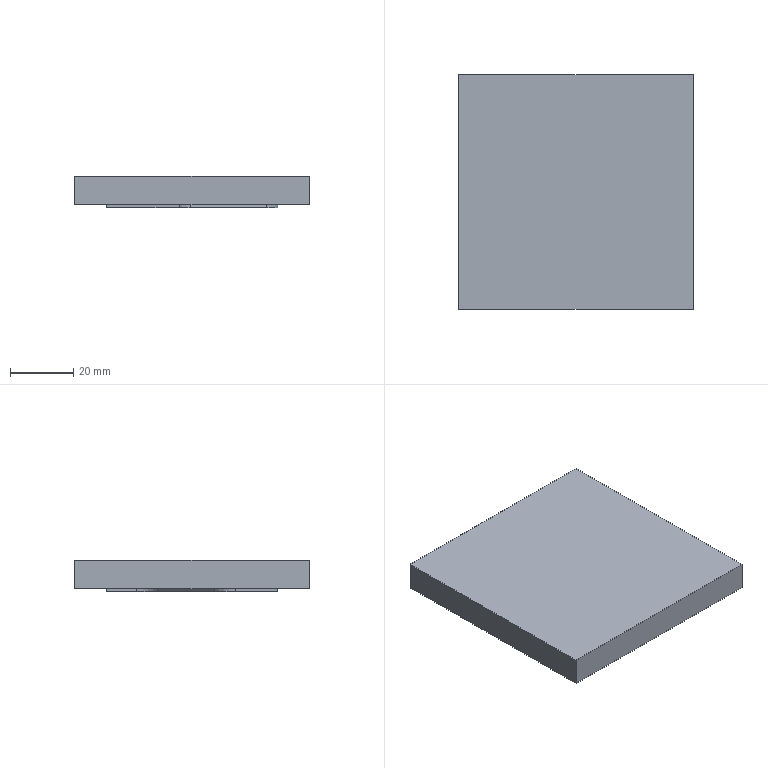NC program | NX | posted with a generic post | part box 74 x 74 x 10 mm
Whole program:
N10 G17 G21 G94 G90
(ZLEVEL_PROFILE_1_COPY_COPY_COPY , TOOL : D1.5)
N12 T19 M6
N14 G54
N16 G17 G0 G90 X3.472 Y4.658 B0. C0. S7500 M3
N18 G43 Z30. H19
N20 Z0.145
N22 G94 G1 X3.468 Y4.656 Z0.108 F1000.
N24 X3.459 Y4.648 Z0.076
N26 X3.445 Y4.635 Z0.047
N28 X3.427 Y4.614 Z0.022
N30 X3.406 Y4.587 Z0.
N32 X3.383 Y4.552 Z-0.019
N34 X3.359 Y4.508 Z-0.035
N36 X3.336 Y4.455 Z-0.048
N38 X3.313 Y4.392 Z-0.059
N40 X3.292 Y4.319 Z-0.067
N42 X3.274 Y4.235 Z-0.073
N44 X3.26 Y4.139 Z-0.077
N46 X3.251 Y4.03 Z-0.079
N48 X3.248 Y3.908 Z-0.08
N50 X3.25 Y2.469 F800.
N52 Y-0.25
N54 X15.75
N56 Y-0.18
N58 Y0.231
N60 X15.701 Y0.254
N62 X14.11 Y0.25
N64 X4.5
N66 G2 X3.75 Y1. R0.75
N68 G1 Y2.5
N70 X3.753 Y3.908
N72 X3.748 Y3.959 Z-0.081
N74 X3.735 Y4.003 Z-0.082
N76 X3.715 Y4.04 Z-0.085
N78 X3.69 Y4.071 Z-0.088
N80 X3.631 Y4.116 Z-0.097
N82 X3.549 Y4.15 Z-0.111
N84 X3.5 Y4.156 Z-0.12
N86 X3.452 Y4.15 Z-0.129
N88 X3.37 Y4.116 Z-0.143
N90 X3.311 Y4.071 Z-0.152
N92 X3.286 Y4.04 Z-0.155
N94 X3.266 Y4.003 Z-0.158
N96 X3.253 Y3.959 Z-0.159
N98 X3.248 Y3.908 Z-0.16
N100 X3.25 Y2.469
N102 Y-0.25
N104 X15.75
N106 Y-0.18
N108 Y0.231
N110 X15.701 Y0.254
N112 X14.11 Y0.25
N114 X4.5
N116 G2 X3.75 Y1. R0.75
N118 G1 Y2.5
N120 X3.753 Y3.908
N122 X3.748 Y3.959 Z-0.161
N124 X3.735 Y4.003 Z-0.162
N126 X3.715 Y4.04 Z-0.165
N128 X3.69 Y4.071 Z-0.168
N130 X3.631 Y4.116 Z-0.177
N132 X3.549 Y4.15 Z-0.191
N134 X3.5 Y4.156 Z-0.2
N136 X3.452 Y4.15 Z-0.209
N138 X3.37 Y4.116 Z-0.223
N140 X3.311 Y4.071 Z-0.232
N142 X3.286 Y4.04 Z-0.235
N144 X3.266 Y4.003 Z-0.238
N146 X3.253 Y3.959 Z-0.239
N148 X3.248 Y3.908 Z-0.24
N150 X3.25 Y2.469
N152 Y-0.25
N154 X15.75
N156 Y-0.18
N158 Y0.231
N160 X15.701 Y0.254
N162 X14.11 Y0.25
N164 X4.5
N166 G2 X3.75 Y1. R0.75
N168 G1 Y2.5
N170 X3.753 Y3.908
N172 X3.748 Y3.959 Z-0.241
N174 X3.735 Y4.003 Z-0.242
N176 X3.715 Y4.04 Z-0.245
N178 X3.69 Y4.071 Z-0.248
N180 X3.631 Y4.116 Z-0.257
N182 X3.549 Y4.15 Z-0.271
N184 X3.5 Y4.156 Z-0.28
N186 X3.452 Y4.15 Z-0.289
N188 X3.37 Y4.116 Z-0.303
N190 X3.311 Y4.071 Z-0.312
N192 X3.286 Y4.04 Z-0.315
N194 X3.266 Y4.003 Z-0.318
N196 X3.253 Y3.959 Z-0.319
N198 X3.248 Y3.908 Z-0.32
N200 X3.25 Y2.469
N202 Y-0.25
N204 X15.75
N206 Y-0.18
N208 Y0.231
N210 X15.701 Y0.254
N212 X14.11 Y0.25
N214 X4.5
N216 G2 X3.75 Y1. R0.75
N218 G1 Y2.5
N220 X3.753 Y3.908
N222 X3.748 Y3.959 Z-0.321
N224 X3.735 Y4.003 Z-0.322
N226 X3.715 Y4.04 Z-0.325
N228 X3.69 Y4.071 Z-0.328
N230 X3.631 Y4.116 Z-0.337
N232 X3.549 Y4.15 Z-0.351
N234 X3.5 Y4.156 Z-0.36
N236 X3.452 Y4.15 Z-0.369
N238 X3.37 Y4.116 Z-0.383
N240 X3.311 Y4.071 Z-0.392
N242 X3.286 Y4.04 Z-0.395
N244 X3.266 Y4.003 Z-0.398
N246 X3.253 Y3.959 Z-0.399
N248 X3.248 Y3.908 Z-0.4
N250 X3.25 Y2.469
N252 Y-0.25
N254 X15.75
N256 Y-0.18
N258 Y0.231
N260 X15.701 Y0.254
N262 X14.11 Y0.25
N264 X4.5
N266 G2 X3.75 Y1. R0.75
N268 G1 Y2.5
N270 X3.753 Y3.908
N272 X3.748 Y3.959 Z-0.401
N274 X3.735 Y4.003 Z-0.402
N276 X3.715 Y4.04 Z-0.405
N278 X3.69 Y4.071 Z-0.408
N280 X3.631 Y4.116 Z-0.417
N282 X3.549 Y4.15 Z-0.431
N284 X3.5 Y4.156 Z-0.44
N286 X3.452 Y4.15 Z-0.449
N288 X3.37 Y4.116 Z-0.463
N290 X3.311 Y4.071 Z-0.472
N292 X3.286 Y4.04 Z-0.475
N294 X3.266 Y4.003 Z-0.478
N296 X3.253 Y3.959 Z-0.479
N298 X3.248 Y3.908 Z-0.48
N300 X3.25 Y2.469
N302 Y-0.25
N304 X15.75
N306 Y-0.18
N308 Y0.231
N310 X15.701 Y0.254
N312 X14.11 Y0.25
N314 X4.5
N316 G2 X3.75 Y1. R0.75
N318 G1 Y2.5
N320 X3.753 Y3.908
N322 X3.748 Y3.959 Z-0.481
N324 X3.735 Y4.003 Z-0.482
N326 X3.715 Y4.04 Z-0.485
N328 X3.69 Y4.071 Z-0.488
N330 X3.631 Y4.116 Z-0.497
N332 X3.549 Y4.15 Z-0.511
N334 X3.5 Y4.156 Z-0.52
N336 X3.452 Y4.15 Z-0.529
N338 X3.37 Y4.116 Z-0.543
N340 X3.311 Y4.071 Z-0.552
N342 X3.286 Y4.04 Z-0.555
N344 X3.266 Y4.003 Z-0.558
N346 X3.253 Y3.959 Z-0.559
N348 X3.248 Y3.908 Z-0.56
N350 X3.25 Y2.469
N352 Y-0.25
N354 X15.75
N356 Y-0.18
N358 Y0.231
N360 X15.701 Y0.254
N362 X14.11 Y0.25
N364 X4.5
N366 G2 X3.75 Y1. R0.75
N368 G1 Y2.5
N370 X3.753 Y3.908
N372 X3.748 Y3.959 Z-0.561
N374 X3.735 Y4.003 Z-0.562
N376 X3.715 Y4.04 Z-0.565
N378 X3.69 Y4.071 Z-0.568
N380 X3.631 Y4.116 Z-0.577
N382 X3.549 Y4.15 Z-0.591
N384 X3.5 Y4.156 Z-0.6
N386 X3.452 Y4.15 Z-0.609
N388 X3.37 Y4.116 Z-0.623
N390 X3.311 Y4.071 Z-0.632
N392 X3.286 Y4.04 Z-0.635
N394 X3.266 Y4.003 Z-0.638
N396 X3.253 Y3.959 Z-0.639
N398 X3.248 Y3.908 Z-0.64
N400 X3.25 Y2.469
N402 Y-0.25
N404 X15.75
N406 Y-0.18
N408 Y0.231
N410 X15.701 Y0.254
N412 X14.11 Y0.25
N414 X4.5
N416 G2 X3.75 Y1. R0.75
N418 G1 Y2.5
N420 X3.753 Y3.908
N422 X3.748 Y3.959 Z-0.641
N424 X3.735 Y4.003 Z-0.642
N426 X3.715 Y4.04 Z-0.645
N428 X3.69 Y4.071 Z-0.648
N430 X3.631 Y4.116 Z-0.657
N432 X3.549 Y4.15 Z-0.671
N434 X3.5 Y4.156 Z-0.68
N436 X3.452 Y4.15 Z-0.689
N438 X3.37 Y4.116 Z-0.703
N440 X3.311 Y4.071 Z-0.712
N442 X3.286 Y4.04 Z-0.715
N444 X3.266 Y4.003 Z-0.718
N446 X3.253 Y3.959 Z-0.719
N448 X3.248 Y3.908 Z-0.72
N450 X3.25 Y2.469
N452 Y-0.25
N454 X15.75
N456 Y-0.18
N458 Y0.231
N460 X15.701 Y0.254
N462 X14.11 Y0.25
N464 X4.5
N466 G2 X3.75 Y1. R0.75
N468 G1 Y2.5
N470 X3.753 Y3.908
N472 X3.748 Y3.959 Z-0.721
N474 X3.735 Y4.003 Z-0.722
N476 X3.715 Y4.04 Z-0.725
N478 X3.69 Y4.071 Z-0.728
N480 X3.631 Y4.116 Z-0.737
N482 X3.549 Y4.15 Z-0.751
N484 X3.5 Y4.156 Z-0.76
N486 X3.452 Y4.15 Z-0.769
N488 X3.37 Y4.116 Z-0.783
N490 X3.311 Y4.071 Z-0.792
N492 X3.286 Y4.04 Z-0.795
N494 X3.266 Y4.003 Z-0.798
N496 X3.253 Y3.959 Z-0.799
N498 X3.248 Y3.908 Z-0.8
N500 X3.25 Y2.469
N502 Y-0.25
N504 X15.75
N506 Y-0.18
N508 Y0.231
N510 X15.701 Y0.253
N512 X14.11 Y0.25
N514 X4.5
N516 G2 X3.75 Y1. R0.75
N518 G1 Y2.5
N520 X3.753 Y3.908
N522 X3.748 Y3.959 Z-0.801
N524 X3.735 Y4.003 Z-0.802
N526 X3.715 Y4.04 Z-0.805
N528 X3.69 Y4.071 Z-0.808
N530 X3.631 Y4.116 Z-0.817
N532 X3.549 Y4.15 Z-0.831
N534 X3.5 Y4.156 Z-0.84
N536 X3.452 Y4.15 Z-0.849
N538 X3.37 Y4.116 Z-0.863
N540 X3.311 Y4.07 Z-0.872
N542 X3.286 Y4.04 Z-0.875
N544 X3.266 Y4.003 Z-0.878
N546 X3.253 Y3.959 Z-0.879
N548 X3.248 Y3.908 Z-0.88
N550 X3.25 Y2.469
N552 Y-0.25
N554 X15.75
N556 Y-0.18
N558 Y0.231
N560 X15.701 Y0.253
N562 X14.11 Y0.25
N564 X4.5
N566 G2 X3.75 Y1. R0.75
N568 G1 Y2.5
N570 X3.753 Y3.908
N572 X3.748 Y3.959 Z-0.881
N574 X3.735 Y4.003 Z-0.882
N576 X3.715 Y4.04 Z-0.885
N578 X3.69 Y4.07 Z-0.888
N580 X3.631 Y4.116 Z-0.897
N582 X3.549 Y4.15 Z-0.911
N584 X3.5 Y4.156 Z-0.92
N586 X3.452 Y4.15 Z-0.929
N588 X3.37 Y4.116 Z-0.943
N590 X3.311 Y4.07 Z-0.952
N592 X3.286 Y4.04 Z-0.955
N594 X3.266 Y4.003 Z-0.958
N596 X3.253 Y3.959 Z-0.959
N598 X3.248 Y3.908 Z-0.96
N600 X3.25 Y2.469
N602 Y-0.25
N604 X15.75
N606 Y-0.18
N608 Y0.231
N610 X15.701 Y0.253
N612 X14.11 Y0.25
N614 X4.5
N616 G2 X3.75 Y1. R0.75
N618 G1 Y2.5
N620 X3.752 Y3.908
N622 X3.748 Y3.959 Z-0.961
N624 X3.735 Y4.003 Z-0.962
N626 X3.715 Y4.04 Z-0.965
N628 X3.69 Y4.07 Z-0.968
N630 X3.631 Y4.116 Z-0.977
N632 X3.549 Y4.15 Z-0.991
N634 X3.5 Y4.156 Z-1.
N636 X3.452 Y4.15 Z-1.009
N638 X3.37 Y4.116 Z-1.023
N640 X3.311 Y4.07 Z-1.032
N642 X3.286 Y4.04 Z-1.035
N644 X3.266 Y4.003 Z-1.038
N646 X3.253 Y3.959 Z-1.039
N648 X3.248 Y3.908 Z-1.04
N650 X3.25 Y2.469
N652 Y-0.25
N654 X15.75
N656 Y-0.18
N658 Y0.231
N660 X15.701 Y0.253
N662 X14.11 Y0.25
N664 X4.5
N666 G2 X3.75 Y1. R0.75
N668 G1 Y2.5
N670 X3.752 Y3.908
N672 X3.748 Y3.959 Z-1.041
N674 X3.735 Y4.003 Z-1.042
N676 X3.715 Y4.04 Z-1.045
N678 X3.69 Y4.07 Z-1.048
N680 X3.631 Y4.116 Z-1.057
N682 X3.549 Y4.15 Z-1.071
N684 X3.5 Y4.155 Z-1.08
N686 X3.452 Y4.15 Z-1.089
N688 X3.37 Y4.116 Z-1.103
N690 X3.311 Y4.07 Z-1.112
N692 X3.286 Y4.04 Z-1.115
N694 X3.266 Y4.003 Z-1.118
N696 X3.253 Y3.959 Z-1.119
N698 X3.248 Y3.908 Z-1.12
N700 X3.25 Y2.469
N702 Y-0.25
N704 X15.75
N706 Y-0.18
N708 Y0.231
N710 X15.701 Y0.253
N712 X14.11 Y0.25
N714 X4.5
N716 G2 X3.75 Y1. R0.75
N718 G1 Y2.5
N720 X3.752 Y3.908
N722 X3.748 Y3.959 Z-1.121
N724 X3.735 Y4.003 Z-1.122
N726 X3.715 Y4.04 Z-1.125
N728 X3.69 Y4.07 Z-1.128
N730 X3.631 Y4.116 Z-1.137
N732 X3.549 Y4.149 Z-1.151
N734 X3.5 Y4.155 Z-1.16
N736 X3.452 Y4.149 Z-1.169
N738 X3.37 Y4.116 Z-1.183
N740 X3.311 Y4.07 Z-1.192
N742 X3.286 Y4.04 Z-1.195
N744 X3.266 Y4.003 Z-1.198
N746 X3.253 Y3.959 Z-1.199
N748 X3.248 Y3.908 Z-1.2
N750 X3.25 Y2.469
N752 Y-0.25
N754 X15.75
N756 Y-0.18
N758 Y0.231
N760 X15.701 Y0.253
N762 X14.11 Y0.25
N764 X4.5
N766 G2 X3.75 Y1. R0.75
N768 G1 Y2.5
N770 X3.752 Y3.908
N772 X3.748 Y3.959 Z-1.201
N774 X3.735 Y4.003 Z-1.202
N776 X3.715 Y4.04 Z-1.205
N778 X3.69 Y4.07 Z-1.208
N780 X3.631 Y4.116 Z-1.217
N782 X3.549 Y4.149 Z-1.231
N784 X3.5 Y4.155 Z-1.24
N786 X3.452 Y4.149 Z-1.249
N788 X3.37 Y4.116 Z-1.263
N790 X3.311 Y4.07 Z-1.272
N792 X3.286 Y4.04 Z-1.275
N794 X3.266 Y4.003 Z-1.278
N796 X3.253 Y3.959 Z-1.279
N798 X3.248 Y3.908 Z-1.28
N800 X3.25 Y2.469
N802 Y-0.25
N804 X15.75
N806 Y-0.18
N808 Y0.231
N810 X15.701 Y0.253
N812 X14.11 Y0.25
N814 X4.5
N816 G2 X3.75 Y1. R0.75
N818 G1 Y2.5
N820 X3.752 Y3.908
N822 X3.748 Y3.959 Z-1.281
N824 X3.735 Y4.003 Z-1.282
N826 X3.715 Y4.04 Z-1.285
N828 X3.69 Y4.07 Z-1.288
N830 X3.631 Y4.116 Z-1.297
N832 X3.549 Y4.149 Z-1.311
N834 X3.5 Y4.155 Z-1.32
N836 X3.452 Y4.149 Z-1.329
N838 X3.37 Y4.116 Z-1.343
N840 X3.311 Y4.07 Z-1.352
N842 X3.286 Y4.04 Z-1.355
N844 X3.266 Y4.003 Z-1.358
N846 X3.253 Y3.959 Z-1.359
N848 X3.248 Y3.908 Z-1.36
N850 X3.25 Y2.469
N852 Y-0.25
N854 X15.75
N856 Y-0.18
N858 Y0.231
N860 X15.701 Y0.253
N862 X14.11 Y0.25
N864 X4.5
N866 G2 X3.75 Y1. R0.75
N868 G1 Y2.5
N870 X3.752 Y3.908
N872 X3.748 Y3.959 Z-1.361
N874 X3.734 Y4.003 Z-1.362
N876 X3.715 Y4.04 Z-1.365
N878 X3.69 Y4.07 Z-1.368
N880 X3.631 Y4.116 Z-1.377
N882 X3.549 Y4.149 Z-1.391
N884 X3.5 Y4.155 Z-1.4
N886 X3.452 Y4.149 Z-1.409
N888 X3.37 Y4.116 Z-1.423
N890 X3.311 Y4.07 Z-1.432
N892 X3.286 Y4.04 Z-1.435
N894 X3.266 Y4.003 Z-1.438
N896 X3.253 Y3.959 Z-1.439
N898 X3.248 Y3.908 Z-1.44
N900 X3.25 Y2.469
N902 Y-0.25
N904 X15.75
N906 Y-0.18
N908 Y0.231
N910 X15.701 Y0.253
N912 X14.11 Y0.25
N914 X4.5
N916 G2 X3.75 Y1. R0.75
N918 G1 Y2.5
N920 X3.752 Y3.908
N922 X3.748 Y3.959 Z-1.441
N924 X3.734 Y4.003 Z-1.442
N926 X3.715 Y4.04 Z-1.445
N928 X3.69 Y4.07 Z-1.448
N930 X3.631 Y4.116 Z-1.457
N932 X3.549 Y4.149 Z-1.471
N934 X3.5 Y4.155 Z-1.48
N936 X3.452 Y4.149 Z-1.489
N938 X3.37 Y4.116 Z-1.503
N940 X3.311 Y4.07 Z-1.512
N942 X3.286 Y4.04 Z-1.515
N944 X3.266 Y4.003 Z-1.518
N946 X3.253 Y3.959 Z-1.519
N948 X3.248 Y3.908 Z-1.52
N950 X3.25 Y2.469
N952 Y-0.25
N954 X15.75
N956 Y-0.18
N958 Y0.231
N960 X15.701 Y0.253
N962 X14.11 Y0.25
N964 X4.5
N966 G2 X3.75 Y1. R0.75
N968 G1 Y2.5
N970 X3.752 Y3.908
N972 X3.748 Y3.959 Z-1.521
N974 X3.734 Y4.003 Z-1.522
N976 X3.715 Y4.04 Z-1.525
N978 X3.689 Y4.07 Z-1.528
N980 X3.631 Y4.116 Z-1.537
N982 X3.549 Y4.149 Z-1.551
N984 X3.5 Y4.155 Z-1.56
N986 X3.452 Y4.149 Z-1.569
N988 X3.37 Y4.116 Z-1.583
N990 X3.311 Y4.07 Z-1.592
N992 X3.286 Y4.04 Z-1.595
N994 X3.266 Y4.003 Z-1.598
N996 X3.253 Y3.959 Z-1.599
N998 X3.248 Y3.908 Z-1.6
N1000 X3.25 Y2.469
N1002 Y-0.25
N1004 X15.75
N1006 Y-0.18
N1008 Y0.231
N1010 X15.701 Y0.253
N1012 X14.11 Y0.25
N1014 X4.5
N1016 G2 X3.75 Y1. R0.75
N1018 G1 Y2.5
N1020 X3.752 Y3.908
N1022 X3.747 Y3.959 Z-1.601
N1024 X3.734 Y4.003 Z-1.602
N1026 X3.714 Y4.04 Z-1.605
N1028 X3.689 Y4.07 Z-1.608
N1030 X3.631 Y4.116 Z-1.617
N1032 X3.549 Y4.149 Z-1.631
N1034 X3.5 Y4.155 Z-1.64
N1036 X3.452 Y4.149 Z-1.649
N1038 X3.37 Y4.116 Z-1.663
N1040 X3.311 Y4.07 Z-1.672
N1042 X3.286 Y4.04 Z-1.675
N1044 X3.266 Y4.003 Z-1.678
N1046 X3.253 Y3.959 Z-1.679
N1048 X3.248 Y3.908 Z-1.68
N1050 X3.25 Y2.469
N1052 Y-0.25
N1054 X15.75
N1056 Y-0.18
N1058 Y0.231
N1060 X15.701 Y0.253
N1062 X14.11 Y0.25
N1064 X4.5
N1066 G2 X3.75 Y1. R0.75
N1068 G1 Y2.5
N1070 X3.752 Y3.908
N1072 X3.747 Y3.959 Z-1.681
N1074 X3.734 Y4.003 Z-1.682
N1076 X3.714 Y4.04 Z-1.685
N1078 X3.689 Y4.07 Z-1.688
N1080 X3.631 Y4.116 Z-1.697
N1082 X3.549 Y4.149 Z-1.711
N1084 X3.5 Y4.155 Z-1.72
N1086 X3.452 Y4.149 Z-1.729
N1088 X3.37 Y4.116 Z-1.743
N1090 X3.311 Y4.07 Z-1.752
N1092 X3.286 Y4.04 Z-1.755
N1094 X3.266 Y4.003 Z-1.758
N1096 X3.253 Y3.959 Z-1.759
N1098 X3.248 Y3.908 Z-1.76
N1100 X3.25 Y2.469
N1102 Y-0.25
N1104 X15.75
N1106 Y-0.18
N1108 Y0.231
N1110 X15.701 Y0.253
N1112 X14.11 Y0.25
N1114 X4.5
N1116 G2 X3.75 Y1. R0.75
N1118 G1 Y2.5
N1120 X3.752 Y3.908
N1122 X3.747 Y3.959 Z-1.761
N1124 X3.734 Y4.003 Z-1.762
N1126 X3.714 Y4.04 Z-1.765
N1128 X3.689 Y4.07 Z-1.768
N1130 X3.63 Y4.116 Z-1.777
N1132 X3.549 Y4.149 Z-1.791
N1134 X3.5 Y4.155 Z-1.8
N1136 X3.452 Y4.149 Z-1.809
N1138 X3.37 Y4.116 Z-1.823
N1140 X3.311 Y4.07 Z-1.832
N1142 X3.286 Y4.039 Z-1.835
N1144 X3.266 Y4.003 Z-1.838
N1146 X3.253 Y3.959 Z-1.839
N1148 X3.249 Y3.908 Z-1.84
N1150 X3.25 Y2.469
N1152 Y-0.25
N1154 X15.75
N1156 Y-0.18
N1158 Y0.231
N1160 X15.701 Y0.253
N1162 X14.11 Y0.25
N1164 X4.5
N1166 G2 X3.75 Y1. R0.75
N1168 G1 Y2.5
N1170 X3.752 Y3.908
N1172 X3.747 Y3.959 Z-1.841
N1174 X3.734 Y4.003 Z-1.842
N1176 X3.714 Y4.04 Z-1.845
N1178 X3.689 Y4.07 Z-1.848
N1180 X3.63 Y4.116 Z-1.857
N1182 X3.549 Y4.149 Z-1.871
N1184 X3.5 Y4.155 Z-1.88
N1186 X3.452 Y4.149 Z-1.889
N1188 X3.37 Y4.116 Z-1.903
N1190 X3.311 Y4.07 Z-1.912
N1192 X3.286 Y4.039 Z-1.915
N1194 X3.266 Y4.003 Z-1.918
N1196 X3.253 Y3.959 Z-1.919
N1198 X3.249 Y3.908 Z-1.92
N1200 X3.25 Y2.469
N1202 Y-0.25
N1204 X15.75
N1206 Y-0.18
N1208 Y0.231
N1210 X15.701 Y0.253
N1212 X14.11 Y0.25
N1214 X4.5
N1216 G2 X3.75 Y1. R0.75
N1218 G1 Y2.5
N1220 X3.752 Y3.908
N1222 X3.747 Y3.959 Z-1.921
N1224 X3.734 Y4.003 Z-1.922
N1226 X3.714 Y4.039 Z-1.925
N1228 X3.689 Y4.07 Z-1.928
N1230 X3.63 Y4.116 Z-1.937
N1232 X3.549 Y4.149 Z-1.951
N1234 X3.5 Y4.155 Z-1.96
N1236 X3.452 Y4.149 Z-1.969
N1238 X3.37 Y4.116 Z-1.983
N1240 X3.311 Y4.07 Z-1.992
N1242 X3.286 Y4.039 Z-1.995
N1244 X3.266 Y4.003 Z-1.998
N1246 X3.253 Y3.959 Z-1.999
N1248 X3.249 Y3.908 Z-2.
N1250 X3.25 Y2.469
N1252 Y-0.25
N1254 X15.75
N1256 Y-0.18
N1258 Y0.231
N1260 X15.701 Y0.253
N1262 X14.11 Y0.25
N1264 X4.5
N1266 G2 X3.75 Y1. R0.75
N1268 G1 Y2.5
N1270 X3.752 Y3.908
N1272 X3.747 Y3.959 Z-2.001
N1274 X3.734 Y4.003 Z-2.002
N1276 X3.714 Y4.039 Z-2.005
N1278 X3.689 Y4.07 Z-2.008
N1280 X3.63 Y4.116 Z-2.017
N1282 X3.549 Y4.149 Z-2.031
N1284 X3.5 Y4.155 Z-2.04
N1286 X3.452 Y4.149 Z-2.049
N1288 X3.37 Y4.116 Z-2.063
N1290 X3.311 Y4.07 Z-2.072
N1292 X3.286 Y4.039 Z-2.075
N1294 X3.266 Y4.003 Z-2.078
N1296 X3.253 Y3.959 Z-2.079
N1298 X3.249 Y3.908 Z-2.08
N1300 X3.25 Y2.469
N1302 Y-0.25
N1304 X15.75
N1306 Y-0.18
N1308 Y0.231
N1310 X15.701 Y0.253
N1312 X14.11 Y0.25
N1314 X4.5
N1316 G2 X3.75 Y1. R0.75
N1318 G1 Y2.5
N1320 X3.752 Y3.908
N1322 X3.747 Y3.959 Z-2.081
N1324 X3.734 Y4.003 Z-2.082
N1326 X3.714 Y4.039 Z-2.085
N1328 X3.689 Y4.07 Z-2.088
N1330 X3.63 Y4.116 Z-2.097
N1332 X3.549 Y4.149 Z-2.111
N1334 X3.5 Y4.155 Z-2.12
N1336 X3.452 Y4.149 Z-2.129
N1338 X3.37 Y4.115 Z-2.143
N1340 X3.311 Y4.07 Z-2.152
N1342 X3.286 Y4.039 Z-2.155
N1344 X3.266 Y4.003 Z-2.158
N1346 X3.253 Y3.959 Z-2.159
N1348 X3.249 Y3.908 Z-2.16
N1350 X3.25 Y2.469
N1352 Y-0.25
N1354 X15.75
N1356 Y-0.18
N1358 Y0.231
N1360 X15.701 Y0.252
N1362 X14.11 Y0.25
N1364 X4.5
N1366 G2 X3.75 Y1. R0.75
N1368 G1 Y2.5
N1370 X3.752 Y3.908
N1372 X3.747 Y3.959 Z-2.161
N1374 X3.734 Y4.003 Z-2.162
N1376 X3.714 Y4.039 Z-2.165
N1378 X3.689 Y4.07 Z-2.168
N1380 X3.63 Y4.115 Z-2.177
N1382 X3.549 Y4.149 Z-2.191
N1384 X3.5 Y4.155 Z-2.2
N1386 X3.452 Y4.149 Z-2.209
N1388 X3.37 Y4.115 Z-2.223
N1390 X3.311 Y4.07 Z-2.232
N1392 X3.286 Y4.039 Z-2.235
N1394 X3.266 Y4.003 Z-2.238
N1396 X3.253 Y3.959 Z-2.239
N1398 X3.249 Y3.908 Z-2.24
N1400 X3.25 Y2.469
N1402 Y-0.25
N1404 X15.75
N1406 Y-0.18
N1408 Y0.231
N1410 X15.701 Y0.252
N1412 X14.11 Y0.25
N1414 X4.5
N1416 G2 X3.75 Y1. R0.75
N1418 G1 Y2.5
N1420 X3.752 Y3.908
N1422 X3.747 Y3.959 Z-2.241
N1424 X3.734 Y4.003 Z-2.242
N1426 X3.714 Y4.039 Z-2.245
N1428 X3.689 Y4.07 Z-2.248
N1430 X3.63 Y4.115 Z-2.257
N1432 X3.549 Y4.149 Z-2.271
N1434 X3.5 Y4.155 Z-2.28
N1436 X3.452 Y4.149 Z-2.289
N1438 X3.37 Y4.115 Z-2.303
N1440 X3.311 Y4.07 Z-2.312
N1442 X3.286 Y4.039 Z-2.315
N1444 X3.267 Y4.003 Z-2.318
N1446 X3.253 Y3.959 Z-2.319
N1448 X3.249 Y3.908 Z-2.32
N1450 X3.25 Y2.469
N1452 Y-0.25
N1454 X15.75
N1456 Y-0.18
N1458 Y0.231
N1460 X15.701 Y0.252
N1462 X14.11 Y0.25
N1464 X4.5
N1466 G2 X3.75 Y1. R0.75
N1468 G1 Y2.5
N1470 X3.752 Y3.908
N1472 X3.747 Y3.959 Z-2.321
N1474 X3.734 Y4.003 Z-2.322
N1476 X3.714 Y4.039 Z-2.325
N1478 X3.689 Y4.07 Z-2.328
N1480 X3.63 Y4.115 Z-2.337
N1482 X3.549 Y4.149 Z-2.351
N1484 X3.5 Y4.155 Z-2.36
N1486 X3.452 Y4.149 Z-2.369
N1488 X3.37 Y4.115 Z-2.383
N1490 X3.311 Y4.07 Z-2.392
N1492 X3.286 Y4.039 Z-2.395
N1494 X3.267 Y4.003 Z-2.398
N1496 X3.253 Y3.959 Z-2.399
N1498 X3.249 Y3.908 Z-2.4
N1500 X3.25 Y2.469
N1502 Y-0.25
N1504 X15.75
N1506 Y-0.18
N1508 Y0.231
N1510 X15.701 Y0.252
N1512 X14.11 Y0.25
N1514 X4.5
N1516 G2 X3.75 Y1. R0.75
N1518 G1 Y2.5
N1520 X3.752 Y3.908
N1522 X3.747 Y3.959 Z-2.401
N1524 X3.734 Y4.003 Z-2.402
N1526 X3.714 Y4.039 Z-2.405
N1528 X3.689 Y4.07 Z-2.408
N1530 X3.63 Y4.115 Z-2.417
N1532 X3.549 Y4.149 Z-2.431
N1534 X3.5 Y4.155 Z-2.44
N1536 X3.452 Y4.149 Z-2.449
N1538 X3.37 Y4.115 Z-2.463
N1540 X3.311 Y4.07 Z-2.472
N1542 X3.286 Y4.039 Z-2.475
N1544 X3.267 Y4.003 Z-2.478
N1546 X3.253 Y3.959 Z-2.479
N1548 X3.249 Y3.908 Z-2.48
N1550 X3.25 Y2.469
N1552 Y-0.25
N1554 X15.75
N1556 Y-0.18
N1558 Y0.231
N1560 X15.701 Y0.252
N1562 X14.11 Y0.25
N1564 X4.5
N1566 G2 X3.75 Y1. R0.75
N1568 G1 Y2.5
N1570 X3.752 Y3.908
N1572 X3.747 Y3.959 Z-2.481
N1574 X3.734 Y4.003 Z-2.482
N1576 X3.714 Y4.039 Z-2.485
N1578 X3.689 Y4.07 Z-2.488
N1580 X3.63 Y4.115 Z-2.497
N1582 X3.549 Y4.149 Z-2.511
N1584 X3.5 Y4.155 Z-2.52
N1586 X3.452 Y4.149 Z-2.529
N1588 X3.37 Y4.115 Z-2.543
N1590 X3.312 Y4.07 Z-2.552
N1592 X3.287 Y4.039 Z-2.555
N1594 X3.267 Y4.003 Z-2.558
N1596 X3.254 Y3.959 Z-2.559
N1598 X3.249 Y3.908 Z-2.56
N1600 X3.25 Y2.469
N1602 Y-0.25
N1604 X15.75
N1606 Y-0.18
N1608 Y0.231
N1610 X15.701 Y0.252
N1612 X14.11 Y0.25
N1614 X4.5
N1616 G2 X3.75 Y1. R0.75
N1618 G1 Y2.5
N1620 X3.752 Y3.908
N1622 X3.747 Y3.959 Z-2.561
N1624 X3.734 Y4.003 Z-2.562
N1626 X3.714 Y4.039 Z-2.565
N1628 X3.689 Y4.07 Z-2.568
N1630 X3.63 Y4.115 Z-2.577
N1632 X3.549 Y4.149 Z-2.591
N1634 X3.5 Y4.155 Z-2.6
N1636 X3.452 Y4.149 Z-2.609
N1638 X3.37 Y4.115 Z-2.623
N1640 X3.312 Y4.07 Z-2.632
N1642 X3.287 Y4.039 Z-2.635
N1644 X3.267 Y4.003 Z-2.638
N1646 X3.254 Y3.959 Z-2.639
N1648 X3.249 Y3.908 Z-2.64
N1650 X3.25 Y2.469
N1652 Y-0.25
N1654 X15.75
N1656 Y-0.18
N1658 Y0.231
N1660 X15.701 Y0.252
N1662 X14.11 Y0.25
N1664 X4.5
N1666 G2 X3.75 Y1. R0.75
N1668 G1 Y2.5
N1670 X3.752 Y3.908
N1672 X3.747 Y3.959 Z-2.641
N1674 X3.734 Y4.003 Z-2.642
N1676 X3.714 Y4.039 Z-2.645
N1678 X3.689 Y4.07 Z-2.648
N1680 X3.63 Y4.115 Z-2.657
N1682 X3.549 Y4.149 Z-2.671
N1684 X3.5 Y4.155 Z-2.68
N1686 X3.452 Y4.149 Z-2.689
N1688 X3.37 Y4.115 Z-2.703
N1690 X3.312 Y4.07 Z-2.712
N1692 X3.287 Y4.039 Z-2.715
N1694 X3.267 Y4.002 Z-2.718
N1696 X3.254 Y3.959 Z-2.719
N1698 X3.249 Y3.908 Z-2.72
N1700 X3.25 Y2.469
N1702 Y-0.25
N1704 X15.75
N1706 Y-0.18
N1708 Y0.231
N1710 X15.701 Y0.252
N1712 X14.11 Y0.25
N1714 X4.5
N1716 G2 X3.75 Y1. R0.75
N1718 G1 Y2.5
N1720 X3.752 Y3.908
N1722 X3.747 Y3.959 Z-2.721
N1724 X3.734 Y4.003 Z-2.722
N1726 X3.714 Y4.039 Z-2.725
N1728 X3.689 Y4.07 Z-2.728
N1730 X3.63 Y4.115 Z-2.737
N1732 X3.549 Y4.149 Z-2.751
N1734 X3.5 Y4.155 Z-2.76
N1736 X3.452 Y4.149 Z-2.769
N1738 X3.37 Y4.115 Z-2.783
N1740 X3.312 Y4.07 Z-2.792
N1742 X3.287 Y4.039 Z-2.795
N1744 X3.267 Y4.002 Z-2.798
N1746 X3.254 Y3.959 Z-2.799
N1748 X3.249 Y3.908 Z-2.8
N1750 X3.25 Y2.469
N1752 Y-0.25
N1754 X15.75
N1756 Y-0.18
N1758 Y0.231
N1760 X15.701 Y0.252
N1762 X14.11 Y0.25
N1764 X4.5
N1766 G2 X3.75 Y1. R0.75
N1768 G1 Y2.5
N1770 X3.751 Y3.908
N1772 X3.747 Y3.959 Z-2.801
N1774 X3.734 Y4.003 Z-2.802
N1776 X3.714 Y4.039 Z-2.805
N1778 X3.689 Y4.07 Z-2.808
N1780 X3.63 Y4.115 Z-2.817
N1782 X3.549 Y4.149 Z-2.831
N1784 X3.5 Y4.155 Z-2.84
N1786 X3.452 Y4.149 Z-2.849
N1788 X3.37 Y4.115 Z-2.863
N1790 X3.312 Y4.07 Z-2.872
N1792 X3.287 Y4.039 Z-2.875
N1794 X3.267 Y4.002 Z-2.878
N1796 X3.254 Y3.959 Z-2.879
N1798 X3.249 Y3.908 Z-2.88
N1800 X3.25 Y2.469
N1802 Y-0.25
N1804 X15.75
N1806 Y-0.18
N1808 Y0.231
N1810 X15.701 Y0.252
N1812 X14.11 Y0.25
N1814 X4.5
N1816 G2 X3.75 Y1. R0.75
N1818 G1 Y2.5
N1820 X3.751 Y3.908
N1822 X3.747 Y3.959 Z-2.881
N1824 X3.734 Y4.003 Z-2.882
N1826 X3.714 Y4.039 Z-2.885
N1828 X3.689 Y4.07 Z-2.888
N1830 X3.63 Y4.115 Z-2.897
N1832 X3.549 Y4.149 Z-2.911
N1834 X3.5 Y4.155 Z-2.92
N1836 X3.452 Y4.149 Z-2.929
N1838 X3.37 Y4.115 Z-2.943
N1840 X3.312 Y4.07 Z-2.952
N1842 X3.287 Y4.039 Z-2.955
N1844 X3.267 Y4.002 Z-2.958
N1846 X3.254 Y3.959 Z-2.959
N1848 X3.249 Y3.908 Z-2.96
N1850 X3.25 Y2.469
N1852 Y-0.25
N1854 X15.75
N1856 Y-0.18
N1858 X15.749 Y0.231
N1860 X15.701 Y0.252
N1862 X14.11 Y0.25
N1864 X4.5
N1866 G2 X3.75 Y1. R0.75
N1868 G1 Y2.5
N1870 X3.751 Y3.908
N1872 X3.747 Y3.959 Z-2.961
N1874 X3.734 Y4.003 Z-2.962
N1876 X3.714 Y4.039 Z-2.965
N1878 X3.689 Y4.07 Z-2.968
N1880 X3.63 Y4.115 Z-2.977
N1882 X3.549 Y4.149 Z-2.991
N1884 X3.5 Y4.155 Z-3.
N1886 X3.452 Y4.149 Z-3.009
N1888 X3.37 Y4.115 Z-3.023
N1890 X3.312 Y4.07 Z-3.032
N1892 X3.287 Y4.039 Z-3.035
N1894 X3.267 Y4.002 Z-3.038
N1896 X3.254 Y3.959 Z-3.039
N1898 X3.249 Y3.908 Z-3.04
N1900 X3.25 Y2.469
N1902 Y-0.25
N1904 X15.75
N1906 Y-0.18
N1908 X15.749 Y0.231
N1910 X15.701 Y0.252
N1912 X14.11 Y0.25
N1914 X4.5
N1916 G2 X3.75 Y1. R0.75
N1918 G1 Y2.5
N1920 X3.751 Y3.908
N1922 X3.747 Y3.959 Z-3.041
N1924 X3.734 Y4.002 Z-3.042
N1926 X3.714 Y4.039 Z-3.045
N1928 X3.689 Y4.07 Z-3.048
N1930 X3.63 Y4.115 Z-3.057
N1932 X3.549 Y4.149 Z-3.071
N1934 X3.5 Y4.155 Z-3.08
N1936 X3.452 Y4.149 Z-3.089
N1938 X3.37 Y4.115 Z-3.103
N1940 X3.312 Y4.07 Z-3.112
N1942 X3.287 Y4.039 Z-3.115
N1944 X3.267 Y4.002 Z-3.118
N1946 X3.254 Y3.959 Z-3.119
N1948 X3.249 Y3.908 Z-3.12
N1950 X3.25 Y2.469
N1952 Y-0.25
N1954 X15.75
N1956 Y-0.18
N1958 X15.749 Y0.231
N1960 X15.701 Y0.252
N1962 X14.11 Y0.25
N1964 X4.5
N1966 G2 X3.75 Y1. R0.75
N1968 G1 Y2.5
N1970 X3.751 Y3.908
N1972 X3.747 Y3.959 Z-3.121
N1974 X3.734 Y4.002 Z-3.122
N1976 X3.714 Y4.039 Z-3.125
N1978 X3.689 Y4.07 Z-3.128
N1980 X3.63 Y4.115 Z-3.137
N1982 X3.549 Y4.149 Z-3.151
N1984 X3.5 Y4.155 Z-3.16
N1986 X3.452 Y4.149 Z-3.169
N1988 X3.37 Y4.115 Z-3.183
N1990 X3.312 Y4.07 Z-3.192
N1992 X3.287 Y4.039 Z-3.195
N1994 X3.267 Y4.002 Z-3.198
N1996 X3.254 Y3.959 Z-3.199
N1998 X3.249 Y3.908 Z-3.2
N2000 X3.25 Y2.469
N2002 Y-0.25
N2004 X15.75
N2006 Y-0.18
N2008 X15.749 Y0.231
N2010 X15.701 Y0.252
N2012 X14.11 Y0.25
N2014 X4.5
N2016 G2 X3.75 Y1. R0.75
N2018 G1 Y2.5
N2020 X3.751 Y3.908
N2022 X3.747 Y3.959 Z-3.201
N2024 X3.733 Y4.002 Z-3.202
N2026 X3.714 Y4.039 Z-3.205
N2028 X3.689 Y4.07 Z-3.208
N2030 X3.63 Y4.115 Z-3.217
N2032 X3.549 Y4.149 Z-3.231
N2034 X3.5 Y4.155 Z-3.24
N2036 X3.452 Y4.149 Z-3.249
N2038 X3.37 Y4.115 Z-3.263
N2040 X3.312 Y4.07 Z-3.272
N2042 X3.287 Y4.039 Z-3.275
N2044 X3.267 Y4.002 Z-3.278
N2046 X3.254 Y3.959 Z-3.279
N2048 X3.249 Y3.908 Z-3.28
N2050 X3.25 Y2.469
N2052 Y-0.25
N2054 X15.75
N2056 Y-0.18
N2058 X15.749 Y0.231
N2060 X15.701 Y0.252
N2062 X14.11 Y0.25
N2064 X4.5
N2066 G2 X3.75 Y1. R0.75
N2068 G1 Y2.5
N2070 X3.751 Y3.908
N2072 X3.747 Y3.959 Z-3.281
N2074 X3.733 Y4.002 Z-3.282
N2076 X3.714 Y4.039 Z-3.285
N2078 X3.689 Y4.07 Z-3.288
N2080 X3.63 Y4.115 Z-3.297
N2082 X3.549 Y4.149 Z-3.311
N2084 X3.5 Y4.155 Z-3.32
N2086 X3.452 Y4.149 Z-3.329
N2088 X3.37 Y4.115 Z-3.343
N2090 X3.312 Y4.07 Z-3.352
N2092 X3.287 Y4.039 Z-3.355
N2094 X3.267 Y4.002 Z-3.358
N2096 X3.254 Y3.959 Z-3.359
N2098 X3.249 Y3.908 Z-3.36
N2100 X3.25 Y2.469
N2102 Y-0.25
N2104 X15.75
N2106 Y-0.18
N2108 X15.749 Y0.231
N2110 X15.701 Y0.252
N2112 X14.11 Y0.25
N2114 X4.5
N2116 G2 X3.75 Y1. R0.75
N2118 G1 Y2.5
N2120 X3.751 Y3.908
N2122 X3.746 Y3.959 Z-3.361
N2124 X3.733 Y4.002 Z-3.362
N2126 X3.714 Y4.039 Z-3.365
N2128 X3.689 Y4.07 Z-3.368
N2130 X3.63 Y4.115 Z-3.377
N2132 X3.549 Y4.149 Z-3.391
N2134 X3.5 Y4.155 Z-3.4
N2136 X3.452 Y4.149 Z-3.409
N2138 X3.37 Y4.115 Z-3.423
N2140 X3.312 Y4.07 Z-3.432
N2142 X3.287 Y4.039 Z-3.435
N2144 X3.267 Y4.002 Z-3.438
N2146 X3.254 Y3.959 Z-3.439
N2148 X3.249 Y3.908 Z-3.44
N2150 X3.25 Y2.469
N2152 Y-0.25
N2154 X15.75
N2156 Y-0.18
N2158 X15.749 Y0.231
N2160 X15.701 Y0.252
N2162 X14.11 Y0.25
N2164 X4.5
N2166 G2 X3.75 Y1. R0.75
N2168 G1 Y2.5
N2170 X3.751 Y3.908
N2172 X3.746 Y3.959 Z-3.441
N2174 X3.733 Y4.002 Z-3.442
N2176 X3.714 Y4.039 Z-3.445
N2178 X3.689 Y4.07 Z-3.448
N2180 X3.63 Y4.115 Z-3.457
N2182 X3.549 Y4.149 Z-3.471
N2184 X3.5 Y4.155 Z-3.48
N2186 X3.452 Y4.149 Z-3.489
N2188 X3.371 Y4.115 Z-3.503
N2190 X3.312 Y4.07 Z-3.512
N2192 X3.287 Y4.039 Z-3.515
N2194 X3.267 Y4.002 Z-3.518
N2196 X3.254 Y3.959 Z-3.519
N2198 X3.249 Y3.908 Z-3.52
N2200 X3.25 Y2.469
N2202 Y-0.25
N2204 X15.75
N2206 Y-0.18
N2208 X15.749 Y0.231
N2210 X15.701 Y0.251
N2212 X14.11 Y0.25
N2214 X4.5
N2216 G2 X3.75 Y1. R0.75
N2218 G1 Y2.5
N2220 X3.751 Y3.908
N2222 X3.746 Y3.959 Z-3.521
N2224 X3.733 Y4.002 Z-3.522
N2226 X3.713 Y4.039 Z-3.525
N2228 X3.689 Y4.07 Z-3.528
N2230 X3.63 Y4.115 Z-3.537
N2232 X3.549 Y4.149 Z-3.551
N2234 X3.5 Y4.154 Z-3.56
N2236 X3.452 Y4.149 Z-3.569
N2238 X3.371 Y4.115 Z-3.583
N2240 X3.312 Y4.07 Z-3.592
N2242 X3.287 Y4.039 Z-3.595
N2244 X3.267 Y4.002 Z-3.598
N2246 X3.254 Y3.959 Z-3.599
N2248 X3.249 Y3.908 Z-3.6
N2250 X3.25 Y2.469
N2252 Y-0.25
N2254 X15.75
N2256 Y-0.18
N2258 X15.749 Y0.231
N2260 X15.701 Y0.251
N2262 X14.11 Y0.25
N2264 X4.5
N2266 G2 X3.75 Y1. R0.75
N2268 G1 Y2.5
N2270 X3.751 Y3.908
N2272 X3.746 Y3.959 Z-3.601
N2274 X3.733 Y4.002 Z-3.602
N2276 X3.713 Y4.039 Z-3.605
N2278 X3.688 Y4.07 Z-3.608
N2280 X3.63 Y4.115 Z-3.617
N2282 X3.549 Y4.149 Z-3.631
N2284 X3.5 Y4.154 Z-3.64
N2286 X3.452 Y4.148 Z-3.649
N2288 X3.371 Y4.115 Z-3.663
N2290 X3.312 Y4.07 Z-3.672
N2292 X3.287 Y4.039 Z-3.675
N2294 X3.267 Y4.002 Z-3.678
N2296 X3.254 Y3.959 Z-3.679
N2298 X3.249 Y3.908 Z-3.68
N2300 X3.25 Y2.469
N2302 Y-0.25
N2304 X15.75
N2306 Y-0.18
N2308 X15.749 Y0.231
N2310 X15.701 Y0.251
N2312 X14.11 Y0.25
N2314 X4.5
N2316 G2 X3.75 Y1. R0.75
N2318 G1 Y2.5
N2320 X3.751 Y3.908
N2322 X3.746 Y3.959 Z-3.681
N2324 X3.733 Y4.002 Z-3.682
N2326 X3.713 Y4.039 Z-3.685
N2328 X3.688 Y4.07 Z-3.688
N2330 X3.63 Y4.115 Z-3.697
N2332 X3.549 Y4.148 Z-3.711
N2334 X3.5 Y4.154 Z-3.72
N2336 X3.452 Y4.148 Z-3.729
N2338 X3.371 Y4.115 Z-3.743
N2340 X3.312 Y4.07 Z-3.752
N2342 X3.287 Y4.039 Z-3.755
N2344 X3.267 Y4.002 Z-3.758
N2346 X3.254 Y3.959 Z-3.759
N2348 X3.249 Y3.908 Z-3.76
N2350 X3.25 Y2.469
N2352 Y-0.25
N2354 X15.75
N2356 Y-0.18
N2358 X15.749 Y0.231
N2360 X15.701 Y0.251
N2362 X14.11 Y0.25
N2364 X4.5
N2366 G2 X3.75 Y1. R0.75
N2368 G1 Y2.5
N2370 X3.751 Y3.908
N2372 X3.746 Y3.959 Z-3.761
N2374 X3.733 Y4.002 Z-3.762
N2376 X3.713 Y4.039 Z-3.765
N2378 X3.688 Y4.07 Z-3.768
N2380 X3.63 Y4.115 Z-3.777
N2382 X3.549 Y4.148 Z-3.791
N2384 X3.5 Y4.154 Z-3.8
N2386 X3.452 Y4.148 Z-3.809
N2388 X3.371 Y4.115 Z-3.823
N2390 X3.312 Y4.07 Z-3.832
N2392 X3.287 Y4.039 Z-3.835
N2394 X3.267 Y4.002 Z-3.838
N2396 X3.254 Y3.959 Z-3.839
N2398 X3.249 Y3.908 Z-3.84
N2400 X3.25 Y2.469
N2402 Y-0.25
N2404 X15.75
N2406 Y-0.18
N2408 X15.749 Y0.231
N2410 X15.701 Y0.251
N2412 X14.11 Y0.25
N2414 X4.5
N2416 G2 X3.75 Y1. R0.75
N2418 G1 Y2.5
N2420 X3.751 Y3.908
N2422 X3.746 Y3.959 Z-3.841
N2424 X3.733 Y4.002 Z-3.842
N2426 X3.713 Y4.039 Z-3.845
N2428 X3.688 Y4.07 Z-3.848
N2430 X3.63 Y4.115 Z-3.857
N2432 X3.549 Y4.148 Z-3.871
N2434 X3.5 Y4.154 Z-3.88
N2436 X3.452 Y4.148 Z-3.889
N2438 X3.371 Y4.115 Z-3.903
N2440 X3.312 Y4.07 Z-3.912
N2442 X3.287 Y4.039 Z-3.915
N2444 X3.267 Y4.002 Z-3.918
N2446 X3.254 Y3.959 Z-3.919
N2448 X3.249 Y3.908 Z-3.92
N2450 X3.25 Y2.469
N2452 Y-0.25
N2454 X15.75
N2456 Y-0.18
N2458 X15.749 Y0.231
N2460 X15.701 Y0.251
N2462 X14.11 Y0.25
N2464 X4.5
N2466 G2 X3.75 Y1. R0.75
N2468 G1 Y2.5
N2470 X3.751 Y3.908
N2472 X3.746 Y3.959 Z-3.921
N2474 X3.733 Y4.002 Z-3.922
N2476 X3.713 Y4.039 Z-3.925
N2478 X3.688 Y4.07 Z-3.928
N2480 X3.629 Y4.115 Z-3.937
N2482 X3.548 Y4.148 Z-3.951
N2484 X3.499 Y4.154 Z-3.96
N2486 X3.451 Y4.148 Z-3.969
N2488 X3.37 Y4.115 Z-3.983
N2490 X3.311 Y4.07 Z-3.992
N2492 X3.286 Y4.039 Z-3.995
N2494 X3.267 Y4.002 Z-3.998
N2496 X3.254 Y3.959 Z-3.999
N2498 X3.249 Y3.908 Z-4.
N2500 X3.258 Y2.807
N2502 X3.263 Y2.751
N2504 X3.206 Y2.752
N2506 G2 X3.25 Y2.5 R0.75
N2508 G1 Y-0.25
N2510 X15.75
N2512 Y-0.18
N2514 X15.749 Y0.231
N2516 X15.701 Y0.251
N2518 X14.11 Y0.25
N2520 X4.5
N2522 G2 X3.75 Y1. R0.75
N2524 G1 Y2.5
N2526 G2 X3.794 Y2.752 R0.75
N2528 G1 X3.738 Y2.751
N2530 X3.744 Y2.807
N2532 X3.751 Y3.908
N2534 X3.749 Y4.022 Z-3.999
N2536 X3.741 Y4.125 Z-3.997
N2538 X3.729 Y4.217 Z-3.994
N2540 X3.714 Y4.298 Z-3.989
N2542 X3.696 Y4.369 Z-3.982
N2544 X3.675 Y4.432 Z-3.973
N2546 X3.653 Y4.485 Z-3.961
N2548 X3.631 Y4.53 Z-3.948
N2550 X3.589 Y4.597 Z-3.913
N2552 X3.57 Y4.621 Z-3.892
N2554 X3.554 Y4.638 Z-3.868
N2556 X3.542 Y4.65 Z-3.84
N2558 X3.534 Y4.656 Z-3.809
N2560 X3.531 Y4.658 Z-3.775
N2562 G0 Z30.
N2564 M5
N2566 M2